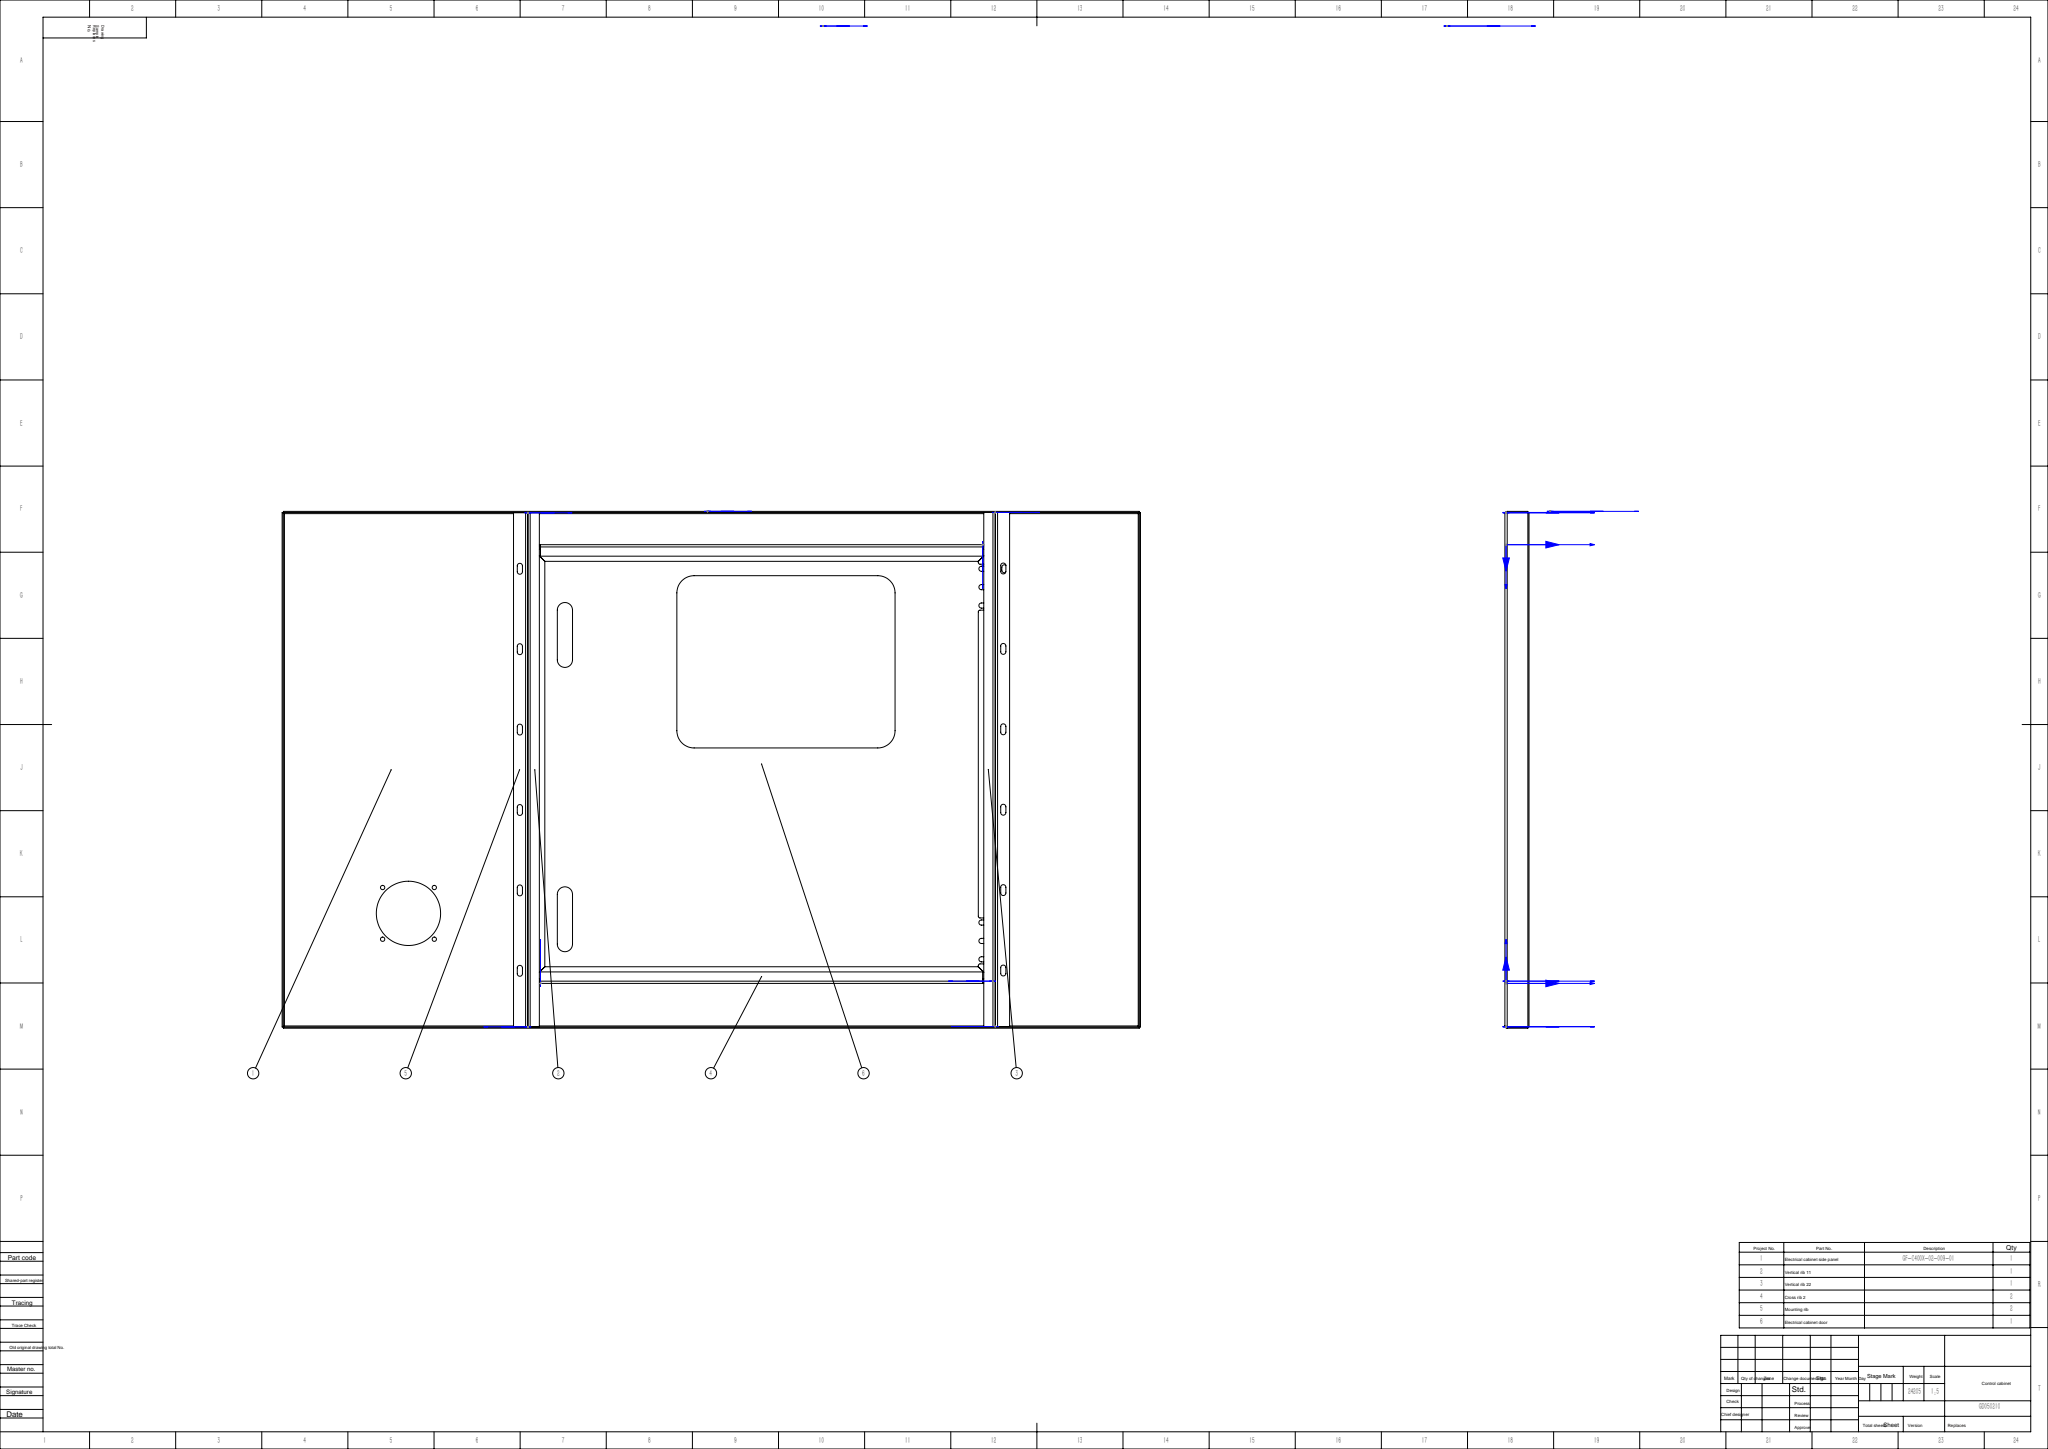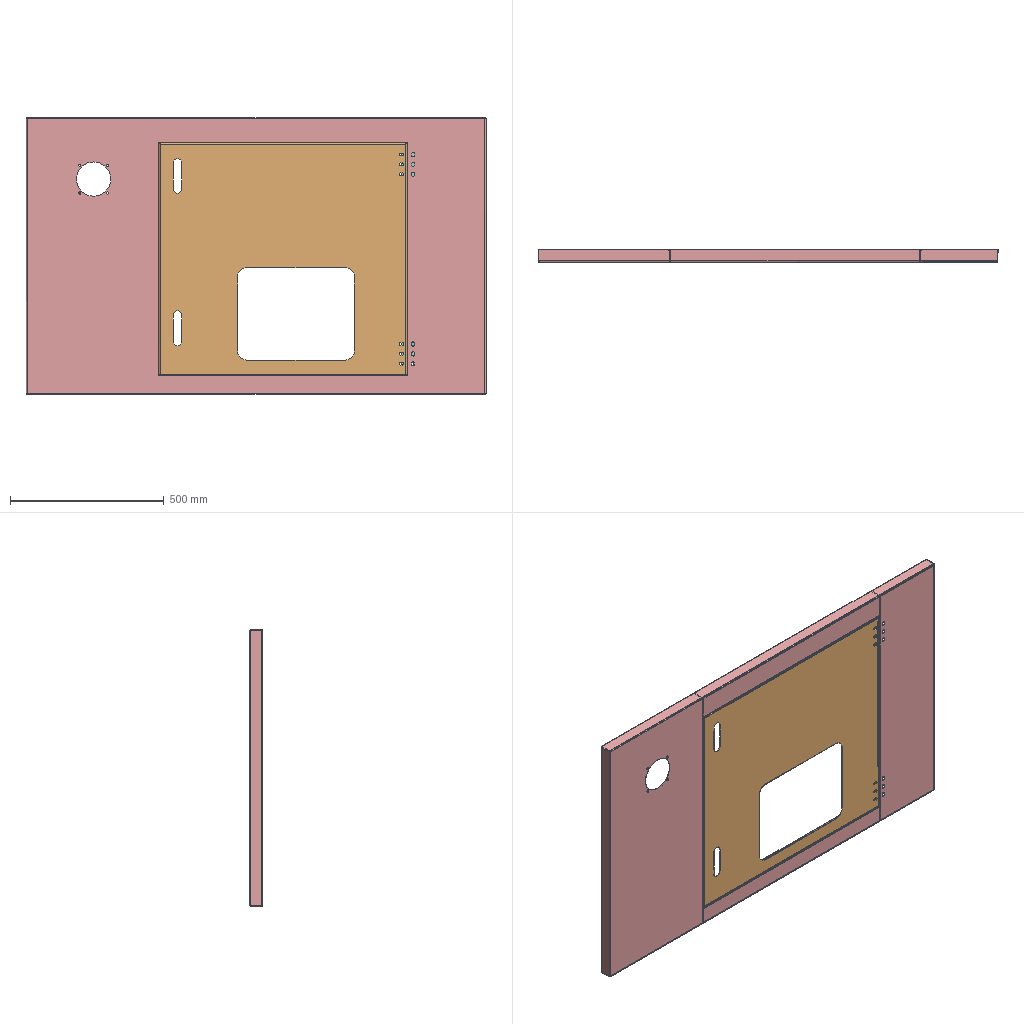Assembly | SolidWorks | 6 different items | 8 placed | box 1495 x 42 x 900 mm
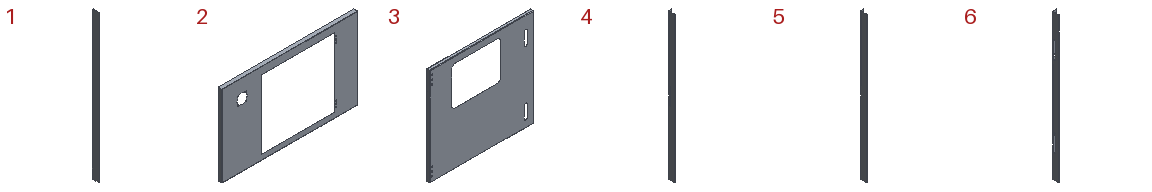Parts list (item | quantity | size | volume | features):
1 | x2 | 20 x 40 x 810 mm | 90217 mm3 | features SMBaseFlange 2, FlatPattern 1, SheetMetal 1
2 | x1 | 1495 x 40 x 900 mm | 1788813 mm3 | features ICE 3, EdgeFlange 1, FlatPattern 1, SMBaseFlange 1, SheetMetal 1
3 | x1 | 805 x 25 x 756 mm | 1238961 mm3 | features CornerFeat 4, ICE 4, EdgeFlange 2, Fillet 2, FlatPattern 1, SMBaseFlange 1, SheetMetal 1
4 | x1 | 20 x 40 x 895 mm | 100259 mm3 | features FlatPattern 1, ICE 1, SMBaseFlange 1, SheetMetal 1
5 | x1 | 20 x 40 x 895 mm | 101515 mm3 | features FlatPattern 1, SMBaseFlange 1, SheetMetal 1
6 | x2 | 25 x 40 x 895 mm | 104308 mm3 | features ICE 2, FlatPattern 1, SMBaseFlange 1, SheetMetal 1
Mates (type | each side: item.copy, entity, surface, feature):
Coincident | 2.1 face plane Base-Flange1 | 4.1 face plane Base-Flange1
Coincident | 2.1 face plane Cut-Extrude1 | 4.1 face plane Base-Flange1
DistanceDim | 4.1 face plane Base-Flange1 | 2.1 face plane Edge-Flange1
Coincident | 2.1 face plane Base-Flange1 | 5.1 face plane Base-Flange1
Coincident | 2.1 face plane Cut-Extrude1 | 5.1 face plane Base-Flange1
Coincident | 2.1 face plane Edge-Flange1 | 5.1 face plane Base-Flange1
Coincident | 2.1 face plane Base-Flange1 | 1.1 face plane Base-Flange1
Coincident | 2.1 face plane Cut-Extrude1 | 1.1 face plane Base-Flange1
Coincident | 4.1 face plane Base-Flange1 | 1.1 face plane Base flange 1
Coincident | 2.1 face plane Base-Flange1 | 1.2 face plane Base-Flange1
Coincident | 2.1 face plane Cut-Extrude1 | 1.2 face plane Base-Flange1
Coincident | 5.1 face plane Base-Flange1 | 1.2 face plane Base flange 1
Coincident | 4.1 face plane Base-Flange1 | 6.1 face plane Base-Flange1 | 2 times
Coincident | 2.1 face plane Base-Flange1 | 6.1 face plane Base-Flange1
Coincident | 5.1 face plane Base-Flange1 | 6.2 face plane Base-Flange1 | 3 times
Coincident | 2.1 face plane Base-Flange1 | 3.1 face plane Base-Flange1
DistanceDim | 3.1 face plane Edge-Flange1 | 5.1 face plane Base-Flange1
DistanceDim | 3.1 face plane Edge-Flange1 | 1.2 face plane Base-Flange1